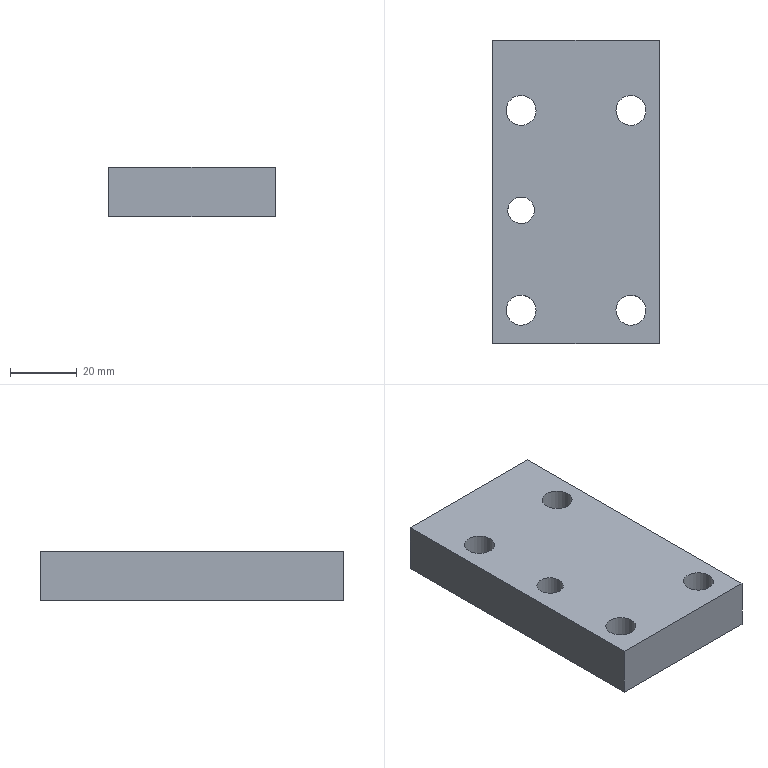Part | STEP file | SN10_006_005-02_PLACA | 1 solid | 11 faces | box 50 x 91 x 15 mm | volume 63679 mm3 | plane 6 | cylinder 5 | commonest cylinder face diameters 9 x4 8 x1
STEP:
#1=CARTESIAN_POINT('',(0.,0.,0.));
#2=DIRECTION('',(0.,0.,1.));
#3=DIRECTION('',(1.,0.,0.));
#4=AXIS2_PLACEMENT_3D('',#1,#2,#3);
#5=CARTESIAN_POINT('',(212.01,-237.918,73.5));
#6=VERTEX_POINT('',#5);
#7=CARTESIAN_POINT('',(208.5,-236.,73.5));
#8=DIRECTION('',(0.,0.,1.));
#9=DIRECTION('',(1.,0.,0.));
#10=AXIS2_PLACEMENT_3D('',#7,#8,#9);
#11=CIRCLE('',#10,4.);
#12=CARTESIAN_POINT('',(208.5,-236.,73.4));
#13=DIRECTION('',(0.,0.,-1.));
#14=DIRECTION('',(0.8776,-0.4794,0.));
#15=AXIS2_PLACEMENT_3D('',#12,#13,#14);
#16=CYLINDRICAL_SURFACE('',#15,4.);
#17=CARTESIAN_POINT('',(12.066,-0.1));
#18=DIRECTION('',(-1.,0.));
#19=VECTOR('',#18,1.);
#20=LINE('',#17,#19);
#21=(GEOMETRIC_REPRESENTATION_CONTEXT(2)PARAMETRIC_REPRESENTATION_CONTEXT()REPRESENTATION_CONTEXT('',''));
#22=DEFINITIONAL_REPRESENTATION('',(#20),#21);
#23=PCURVE('',#16,#22);
#24=CARTESIAN_POINT('',(200.,-185.,73.5));
#25=DIRECTION('',(0.,0.,1.));
#26=DIRECTION('',(1.,0.,0.));
#27=AXIS2_PLACEMENT_3D('',#24,#25,#26);
#28=PLANE('',#27);
#29=CARTESIAN_POINT('',(8.5,-51.));
#30=DIRECTION('',(1.,0.));
#31=AXIS2_PLACEMENT_2D('',#29,#30);
#32=CIRCLE('',#31,4.);
#33=(GEOMETRIC_REPRESENTATION_CONTEXT(2)PARAMETRIC_REPRESENTATION_CONTEXT()REPRESENTATION_CONTEXT('',''));
#34=DEFINITIONAL_REPRESENTATION('',(#32),#33);
#35=PCURVE('',#28,#34);
#36=SURFACE_CURVE('',#11,(#23,#35),.PCURVE_S1.);
#37=EDGE_CURVE('',#6,#6,#36,.T.);
#38=ORIENTED_EDGE('',*,*,#37,.F.);
#39=CARTESIAN_POINT('',(212.01,-237.918,58.5));
#40=VERTEX_POINT('',#39);
#41=CARTESIAN_POINT('',(212.01,-237.918,73.5));
#42=CARTESIAN_POINT('',(212.01,-237.918,58.5));
#43=B_SPLINE_CURVE_WITH_KNOTS('',1,(#41,#42),.UNSPECIFIED.,.F.,.F.,(2,2),(-0.1,14.9),.PIECEWISE_BEZIER_KNOTS.);
#44=CARTESIAN_POINT('',(6.283,0.));
#45=DIRECTION('',(0.,1.));
#46=VECTOR('',#45,1.);
#47=LINE('',#44,#46);
#48=(GEOMETRIC_REPRESENTATION_CONTEXT(2)PARAMETRIC_REPRESENTATION_CONTEXT()REPRESENTATION_CONTEXT('',''));
#49=DEFINITIONAL_REPRESENTATION('',(#47),#48);
#50=PCURVE('',#16,#49);
#51=CARTESIAN_POINT('',(0.,0.));
#52=DIRECTION('',(0.,1.));
#53=VECTOR('',#52,1.);
#54=LINE('',#51,#53);
#55=(GEOMETRIC_REPRESENTATION_CONTEXT(2)PARAMETRIC_REPRESENTATION_CONTEXT()REPRESENTATION_CONTEXT('',''));
#56=DEFINITIONAL_REPRESENTATION('',(#54),#55);
#57=PCURVE('',#16,#56);
#58=SEAM_CURVE('',#43,(#50,#57),.PCURVE_S1.);
#59=EDGE_CURVE('',#6,#40,#58,.T.);
#60=ORIENTED_EDGE('',*,*,#59,.T.);
#61=CARTESIAN_POINT('',(208.5,-236.,58.5));
#62=DIRECTION('',(0.,0.,-1.));
#63=DIRECTION('',(1.,0.,0.));
#64=AXIS2_PLACEMENT_3D('',#61,#62,#63);
#65=CIRCLE('',#64,4.);
#66=CARTESIAN_POINT('',(-0.5,14.9));
#67=DIRECTION('',(1.,0.));
#68=VECTOR('',#67,1.);
#69=LINE('',#66,#68);
#70=(GEOMETRIC_REPRESENTATION_CONTEXT(2)PARAMETRIC_REPRESENTATION_CONTEXT()REPRESENTATION_CONTEXT('',''));
#71=DEFINITIONAL_REPRESENTATION('',(#69),#70);
#72=PCURVE('',#16,#71);
#73=CARTESIAN_POINT('',(200.,-276.,58.5));
#74=DIRECTION('',(0.,0.,-1.));
#75=DIRECTION('',(-1.,0.,0.));
#76=AXIS2_PLACEMENT_3D('',#73,#74,#75);
#77=PLANE('',#76);
#78=CARTESIAN_POINT('',(-8.5,40.));
#79=DIRECTION('',(-1.,0.));
#80=AXIS2_PLACEMENT_2D('',#78,#79);
#81=CIRCLE('',#80,4.);
#82=(GEOMETRIC_REPRESENTATION_CONTEXT(2)PARAMETRIC_REPRESENTATION_CONTEXT()REPRESENTATION_CONTEXT('',''));
#83=DEFINITIONAL_REPRESENTATION('',(#81),#82);
#84=PCURVE('',#77,#83);
#85=SURFACE_CURVE('',#65,(#72,#84),.PCURVE_S1.);
#86=EDGE_CURVE('',#40,#40,#85,.T.);
#87=ORIENTED_EDGE('',*,*,#86,.F.);
#88=ORIENTED_EDGE('',*,*,#59,.F.);
#89=EDGE_LOOP('',(#38,#60,#87,#88));
#90=FACE_BOUND('',#89,.F.);
#91=ADVANCED_FACE('',(#90),#16,.F.);
#92=CARTESIAN_POINT('',(250.,-185.,73.5));
#93=VERTEX_POINT('',#92);
#94=CARTESIAN_POINT('',(250.,-276.,73.5));
#95=VERTEX_POINT('',#94);
#96=CARTESIAN_POINT('',(250.,-185.,73.5));
#97=DIRECTION('',(0.,-1.,0.));
#98=VECTOR('',#97,1.);
#99=LINE('',#96,#98);
#100=CARTESIAN_POINT('',(50.,0.));
#101=DIRECTION('',(0.,-1.));
#102=VECTOR('',#101,1.);
#103=LINE('',#100,#102);
#104=(GEOMETRIC_REPRESENTATION_CONTEXT(2)PARAMETRIC_REPRESENTATION_CONTEXT()REPRESENTATION_CONTEXT('',''));
#105=DEFINITIONAL_REPRESENTATION('',(#103),#104);
#106=PCURVE('',#28,#105);
#107=CARTESIAN_POINT('',(250.,0.,0.));
#108=DIRECTION('',(-1.,0.,0.));
#109=DIRECTION('',(0.,0.,1.));
#110=AXIS2_PLACEMENT_3D('',#107,#108,#109);
#111=PLANE('',#110);
#112=CARTESIAN_POINT('',(73.5,-185.));
#113=DIRECTION('',(0.,-1.));
#114=VECTOR('',#113,1.);
#115=LINE('',#112,#114);
#116=(GEOMETRIC_REPRESENTATION_CONTEXT(2)PARAMETRIC_REPRESENTATION_CONTEXT()REPRESENTATION_CONTEXT('',''));
#117=DEFINITIONAL_REPRESENTATION('',(#115),#116);
#118=PCURVE('',#111,#117);
#119=SURFACE_CURVE('',#99,(#106,#118),.PCURVE_S1.);
#120=EDGE_CURVE('',#93,#95,#119,.T.);
#121=ORIENTED_EDGE('',*,*,#120,.F.);
#122=CARTESIAN_POINT('',(200.,-185.,73.5));
#123=VERTEX_POINT('',#122);
#124=CARTESIAN_POINT('',(200.,-185.,73.5));
#125=DIRECTION('',(1.,0.,0.));
#126=VECTOR('',#125,1.);
#127=LINE('',#124,#126);
#128=CARTESIAN_POINT('',(0.,0.));
#129=DIRECTION('',(1.,0.));
#130=VECTOR('',#129,1.);
#131=LINE('',#128,#130);
#132=(GEOMETRIC_REPRESENTATION_CONTEXT(2)PARAMETRIC_REPRESENTATION_CONTEXT()REPRESENTATION_CONTEXT('',''));
#133=DEFINITIONAL_REPRESENTATION('',(#131),#132);
#134=PCURVE('',#28,#133);
#135=CARTESIAN_POINT('',(200.,-185.,73.5));
#136=DIRECTION('',(0.,-1.,0.));
#137=DIRECTION('',(0.,0.,-1.));
#138=AXIS2_PLACEMENT_3D('',#135,#136,#137);
#139=PLANE('',#138);
#140=CARTESIAN_POINT('',(0.,0.));
#141=DIRECTION('',(0.,1.));
#142=VECTOR('',#141,1.);
#143=LINE('',#140,#142);
#144=(GEOMETRIC_REPRESENTATION_CONTEXT(2)PARAMETRIC_REPRESENTATION_CONTEXT()REPRESENTATION_CONTEXT('',''));
#145=DEFINITIONAL_REPRESENTATION('',(#143),#144);
#146=PCURVE('',#139,#145);
#147=SURFACE_CURVE('',#127,(#134,#146),.PCURVE_S1.);
#148=EDGE_CURVE('',#123,#93,#147,.T.);
#149=ORIENTED_EDGE('',*,*,#148,.F.);
#150=CARTESIAN_POINT('',(200.,-276.,73.5));
#151=VERTEX_POINT('',#150);
#152=CARTESIAN_POINT('',(200.,-185.,73.5));
#153=DIRECTION('',(0.,-1.,0.));
#154=VECTOR('',#153,1.);
#155=LINE('',#152,#154);
#156=CARTESIAN_POINT('',(0.,0.));
#157=DIRECTION('',(0.,-1.));
#158=VECTOR('',#157,1.);
#159=LINE('',#156,#158);
#160=(GEOMETRIC_REPRESENTATION_CONTEXT(2)PARAMETRIC_REPRESENTATION_CONTEXT()REPRESENTATION_CONTEXT('',''));
#161=DEFINITIONAL_REPRESENTATION('',(#159),#160);
#162=PCURVE('',#28,#161);
#163=CARTESIAN_POINT('',(200.,0.,0.));
#164=DIRECTION('',(-1.,0.,0.));
#165=DIRECTION('',(0.,0.,1.));
#166=AXIS2_PLACEMENT_3D('',#163,#164,#165);
#167=PLANE('',#166);
#168=CARTESIAN_POINT('',(73.5,-185.));
#169=DIRECTION('',(0.,-1.));
#170=VECTOR('',#169,1.);
#171=LINE('',#168,#170);
#172=(GEOMETRIC_REPRESENTATION_CONTEXT(2)PARAMETRIC_REPRESENTATION_CONTEXT()REPRESENTATION_CONTEXT('',''));
#173=DEFINITIONAL_REPRESENTATION('',(#171),#172);
#174=PCURVE('',#167,#173);
#175=SURFACE_CURVE('',#155,(#162,#174),.PCURVE_S1.);
#176=EDGE_CURVE('',#123,#151,#175,.T.);
#177=ORIENTED_EDGE('',*,*,#176,.T.);
#178=CARTESIAN_POINT('',(200.,-276.,73.5));
#179=DIRECTION('',(1.,0.,0.));
#180=VECTOR('',#179,1.);
#181=LINE('',#178,#180);
#182=CARTESIAN_POINT('',(0.,-91.));
#183=DIRECTION('',(1.,0.));
#184=VECTOR('',#183,1.);
#185=LINE('',#182,#184);
#186=(GEOMETRIC_REPRESENTATION_CONTEXT(2)PARAMETRIC_REPRESENTATION_CONTEXT()REPRESENTATION_CONTEXT('',''));
#187=DEFINITIONAL_REPRESENTATION('',(#185),#186);
#188=PCURVE('',#28,#187);
#189=CARTESIAN_POINT('',(200.,-276.,58.5));
#190=DIRECTION('',(0.,1.,0.));
#191=DIRECTION('',(0.,0.,1.));
#192=AXIS2_PLACEMENT_3D('',#189,#190,#191);
#193=PLANE('',#192);
#194=CARTESIAN_POINT('',(15.,0.));
#195=DIRECTION('',(0.,1.));
#196=VECTOR('',#195,1.);
#197=LINE('',#194,#196);
#198=(GEOMETRIC_REPRESENTATION_CONTEXT(2)PARAMETRIC_REPRESENTATION_CONTEXT()REPRESENTATION_CONTEXT('',''));
#199=DEFINITIONAL_REPRESENTATION('',(#197),#198);
#200=PCURVE('',#193,#199);
#201=SURFACE_CURVE('',#181,(#188,#200),.PCURVE_S1.);
#202=EDGE_CURVE('',#151,#95,#201,.T.);
#203=ORIENTED_EDGE('',*,*,#202,.T.);
#204=EDGE_LOOP('',(#121,#149,#177,#203));
#205=FACE_BOUND('',#204,.T.);
#206=ORIENTED_EDGE('',*,*,#37,.F.);
#207=EDGE_LOOP('',(#206));
#208=FACE_BOUND('',#207,.T.);
#209=CARTESIAN_POINT('',(212.449,-268.157,73.5));
#210=VERTEX_POINT('',#209);
#211=CARTESIAN_POINT('',(208.5,-266.,73.5));
#212=DIRECTION('',(0.,0.,1.));
#213=DIRECTION('',(1.,0.,0.));
#214=AXIS2_PLACEMENT_3D('',#211,#212,#213);
#215=CIRCLE('',#214,4.5);
#216=CARTESIAN_POINT('',(8.5,-81.));
#217=DIRECTION('',(1.,0.));
#218=AXIS2_PLACEMENT_2D('',#216,#217);
#219=CIRCLE('',#218,4.5);
#220=(GEOMETRIC_REPRESENTATION_CONTEXT(2)PARAMETRIC_REPRESENTATION_CONTEXT()REPRESENTATION_CONTEXT('',''));
#221=DEFINITIONAL_REPRESENTATION('',(#219),#220);
#222=PCURVE('',#28,#221);
#223=CARTESIAN_POINT('',(208.5,-266.,73.4));
#224=DIRECTION('',(0.,0.,-1.));
#225=DIRECTION('',(0.8776,-0.4794,0.));
#226=AXIS2_PLACEMENT_3D('',#223,#224,#225);
#227=CYLINDRICAL_SURFACE('',#226,4.5);
#228=CARTESIAN_POINT('',(12.066,-0.1));
#229=DIRECTION('',(-1.,0.));
#230=VECTOR('',#229,1.);
#231=LINE('',#228,#230);
#232=(GEOMETRIC_REPRESENTATION_CONTEXT(2)PARAMETRIC_REPRESENTATION_CONTEXT()REPRESENTATION_CONTEXT('',''));
#233=DEFINITIONAL_REPRESENTATION('',(#231),#232);
#234=PCURVE('',#227,#233);
#235=SURFACE_CURVE('',#215,(#222,#234),.PCURVE_S1.);
#236=EDGE_CURVE('',#210,#210,#235,.T.);
#237=ORIENTED_EDGE('',*,*,#236,.F.);
#238=EDGE_LOOP('',(#237));
#239=FACE_BOUND('',#238,.T.);
#240=CARTESIAN_POINT('',(212.449,-208.157,73.5));
#241=VERTEX_POINT('',#240);
#242=CARTESIAN_POINT('',(208.5,-206.,73.5));
#243=DIRECTION('',(0.,0.,1.));
#244=DIRECTION('',(1.,0.,0.));
#245=AXIS2_PLACEMENT_3D('',#242,#243,#244);
#246=CIRCLE('',#245,4.5);
#247=CARTESIAN_POINT('',(8.5,-21.));
#248=DIRECTION('',(1.,0.));
#249=AXIS2_PLACEMENT_2D('',#247,#248);
#250=CIRCLE('',#249,4.5);
#251=(GEOMETRIC_REPRESENTATION_CONTEXT(2)PARAMETRIC_REPRESENTATION_CONTEXT()REPRESENTATION_CONTEXT('',''));
#252=DEFINITIONAL_REPRESENTATION('',(#250),#251);
#253=PCURVE('',#28,#252);
#254=CARTESIAN_POINT('',(208.5,-206.,73.4));
#255=DIRECTION('',(0.,0.,-1.));
#256=DIRECTION('',(0.8776,-0.4794,0.));
#257=AXIS2_PLACEMENT_3D('',#254,#255,#256);
#258=CYLINDRICAL_SURFACE('',#257,4.5);
#259=CARTESIAN_POINT('',(12.066,-0.1));
#260=DIRECTION('',(-1.,0.));
#261=VECTOR('',#260,1.);
#262=LINE('',#259,#261);
#263=(GEOMETRIC_REPRESENTATION_CONTEXT(2)PARAMETRIC_REPRESENTATION_CONTEXT()REPRESENTATION_CONTEXT('',''));
#264=DEFINITIONAL_REPRESENTATION('',(#262),#263);
#265=PCURVE('',#258,#264);
#266=SURFACE_CURVE('',#246,(#253,#265),.PCURVE_S1.);
#267=EDGE_CURVE('',#241,#241,#266,.T.);
#268=ORIENTED_EDGE('',*,*,#267,.F.);
#269=EDGE_LOOP('',(#268));
#270=FACE_BOUND('',#269,.T.);
#271=CARTESIAN_POINT('',(245.449,-268.157,73.5));
#272=VERTEX_POINT('',#271);
#273=CARTESIAN_POINT('',(241.5,-266.,73.5));
#274=DIRECTION('',(0.,0.,1.));
#275=DIRECTION('',(1.,0.,0.));
#276=AXIS2_PLACEMENT_3D('',#273,#274,#275);
#277=CIRCLE('',#276,4.5);
#278=CARTESIAN_POINT('',(41.5,-81.));
#279=DIRECTION('',(1.,0.));
#280=AXIS2_PLACEMENT_2D('',#278,#279);
#281=CIRCLE('',#280,4.5);
#282=(GEOMETRIC_REPRESENTATION_CONTEXT(2)PARAMETRIC_REPRESENTATION_CONTEXT()REPRESENTATION_CONTEXT('',''));
#283=DEFINITIONAL_REPRESENTATION('',(#281),#282);
#284=PCURVE('',#28,#283);
#285=CARTESIAN_POINT('',(241.5,-266.,73.4));
#286=DIRECTION('',(0.,0.,-1.));
#287=DIRECTION('',(0.8776,-0.4794,0.));
#288=AXIS2_PLACEMENT_3D('',#285,#286,#287);
#289=CYLINDRICAL_SURFACE('',#288,4.5);
#290=CARTESIAN_POINT('',(12.066,-0.1));
#291=DIRECTION('',(-1.,0.));
#292=VECTOR('',#291,1.);
#293=LINE('',#290,#292);
#294=(GEOMETRIC_REPRESENTATION_CONTEXT(2)PARAMETRIC_REPRESENTATION_CONTEXT()REPRESENTATION_CONTEXT('',''));
#295=DEFINITIONAL_REPRESENTATION('',(#293),#294);
#296=PCURVE('',#289,#295);
#297=SURFACE_CURVE('',#277,(#284,#296),.PCURVE_S1.);
#298=EDGE_CURVE('',#272,#272,#297,.T.);
#299=ORIENTED_EDGE('',*,*,#298,.F.);
#300=EDGE_LOOP('',(#299));
#301=FACE_BOUND('',#300,.T.);
#302=CARTESIAN_POINT('',(245.449,-208.157,73.5));
#303=VERTEX_POINT('',#302);
#304=CARTESIAN_POINT('',(241.5,-206.,73.5));
#305=DIRECTION('',(0.,0.,1.));
#306=DIRECTION('',(1.,0.,0.));
#307=AXIS2_PLACEMENT_3D('',#304,#305,#306);
#308=CIRCLE('',#307,4.5);
#309=CARTESIAN_POINT('',(41.5,-21.));
#310=DIRECTION('',(1.,0.));
#311=AXIS2_PLACEMENT_2D('',#309,#310);
#312=CIRCLE('',#311,4.5);
#313=(GEOMETRIC_REPRESENTATION_CONTEXT(2)PARAMETRIC_REPRESENTATION_CONTEXT()REPRESENTATION_CONTEXT('',''));
#314=DEFINITIONAL_REPRESENTATION('',(#312),#313);
#315=PCURVE('',#28,#314);
#316=CARTESIAN_POINT('',(241.5,-206.,73.4));
#317=DIRECTION('',(0.,0.,-1.));
#318=DIRECTION('',(0.8776,-0.4794,0.));
#319=AXIS2_PLACEMENT_3D('',#316,#317,#318);
#320=CYLINDRICAL_SURFACE('',#319,4.5);
#321=CARTESIAN_POINT('',(12.066,-0.1));
#322=DIRECTION('',(-1.,0.));
#323=VECTOR('',#322,1.);
#324=LINE('',#321,#323);
#325=(GEOMETRIC_REPRESENTATION_CONTEXT(2)PARAMETRIC_REPRESENTATION_CONTEXT()REPRESENTATION_CONTEXT('',''));
#326=DEFINITIONAL_REPRESENTATION('',(#324),#325);
#327=PCURVE('',#320,#326);
#328=SURFACE_CURVE('',#308,(#315,#327),.PCURVE_S1.);
#329=EDGE_CURVE('',#303,#303,#328,.T.);
#330=ORIENTED_EDGE('',*,*,#329,.F.);
#331=EDGE_LOOP('',(#330));
#332=FACE_BOUND('',#331,.T.);
#333=ADVANCED_FACE('',(#205,#208,#239,#270,#301,#332),#28,.T.);
#334=CARTESIAN_POINT('',(250.,-276.,58.5));
#335=VERTEX_POINT('',#334);
#336=CARTESIAN_POINT('',(250.,-185.,58.5));
#337=VERTEX_POINT('',#336);
#338=CARTESIAN_POINT('',(250.,-276.,58.5));
#339=DIRECTION('',(0.,1.,0.));
#340=VECTOR('',#339,1.);
#341=LINE('',#338,#340);
#342=CARTESIAN_POINT('',(-50.,0.));
#343=DIRECTION('',(0.,1.));
#344=VECTOR('',#343,1.);
#345=LINE('',#342,#344);
#346=(GEOMETRIC_REPRESENTATION_CONTEXT(2)PARAMETRIC_REPRESENTATION_CONTEXT()REPRESENTATION_CONTEXT('',''));
#347=DEFINITIONAL_REPRESENTATION('',(#345),#346);
#348=PCURVE('',#77,#347);
#349=CARTESIAN_POINT('',(58.5,-276.));
#350=DIRECTION('',(0.,1.));
#351=VECTOR('',#350,1.);
#352=LINE('',#349,#351);
#353=(GEOMETRIC_REPRESENTATION_CONTEXT(2)PARAMETRIC_REPRESENTATION_CONTEXT()REPRESENTATION_CONTEXT('',''));
#354=DEFINITIONAL_REPRESENTATION('',(#352),#353);
#355=PCURVE('',#111,#354);
#356=SURFACE_CURVE('',#341,(#348,#355),.PCURVE_S1.);
#357=EDGE_CURVE('',#335,#337,#356,.T.);
#358=ORIENTED_EDGE('',*,*,#357,.F.);
#359=CARTESIAN_POINT('',(200.,-276.,58.5));
#360=VERTEX_POINT('',#359);
#361=CARTESIAN_POINT('',(200.,-276.,58.5));
#362=DIRECTION('',(1.,0.,0.));
#363=VECTOR('',#362,1.);
#364=LINE('',#361,#363);
#365=CARTESIAN_POINT('',(0.,0.));
#366=DIRECTION('',(-1.,0.));
#367=VECTOR('',#366,1.);
#368=LINE('',#365,#367);
#369=(GEOMETRIC_REPRESENTATION_CONTEXT(2)PARAMETRIC_REPRESENTATION_CONTEXT()REPRESENTATION_CONTEXT('',''));
#370=DEFINITIONAL_REPRESENTATION('',(#368),#369);
#371=PCURVE('',#77,#370);
#372=CARTESIAN_POINT('',(0.,0.));
#373=DIRECTION('',(0.,1.));
#374=VECTOR('',#373,1.);
#375=LINE('',#372,#374);
#376=(GEOMETRIC_REPRESENTATION_CONTEXT(2)PARAMETRIC_REPRESENTATION_CONTEXT()REPRESENTATION_CONTEXT('',''));
#377=DEFINITIONAL_REPRESENTATION('',(#375),#376);
#378=PCURVE('',#193,#377);
#379=SURFACE_CURVE('',#364,(#371,#378),.PCURVE_S1.);
#380=EDGE_CURVE('',#360,#335,#379,.T.);
#381=ORIENTED_EDGE('',*,*,#380,.F.);
#382=CARTESIAN_POINT('',(200.,-185.,58.5));
#383=VERTEX_POINT('',#382);
#384=CARTESIAN_POINT('',(200.,-276.,58.5));
#385=DIRECTION('',(0.,1.,0.));
#386=VECTOR('',#385,1.);
#387=LINE('',#384,#386);
#388=CARTESIAN_POINT('',(0.,0.));
#389=DIRECTION('',(0.,1.));
#390=VECTOR('',#389,1.);
#391=LINE('',#388,#390);
#392=(GEOMETRIC_REPRESENTATION_CONTEXT(2)PARAMETRIC_REPRESENTATION_CONTEXT()REPRESENTATION_CONTEXT('',''));
#393=DEFINITIONAL_REPRESENTATION('',(#391),#392);
#394=PCURVE('',#77,#393);
#395=CARTESIAN_POINT('',(58.5,-276.));
#396=DIRECTION('',(0.,1.));
#397=VECTOR('',#396,1.);
#398=LINE('',#395,#397);
#399=(GEOMETRIC_REPRESENTATION_CONTEXT(2)PARAMETRIC_REPRESENTATION_CONTEXT()REPRESENTATION_CONTEXT('',''));
#400=DEFINITIONAL_REPRESENTATION('',(#398),#399);
#401=PCURVE('',#167,#400);
#402=SURFACE_CURVE('',#387,(#394,#401),.PCURVE_S1.);
#403=EDGE_CURVE('',#360,#383,#402,.T.);
#404=ORIENTED_EDGE('',*,*,#403,.T.);
#405=CARTESIAN_POINT('',(200.,-185.,58.5));
#406=DIRECTION('',(1.,0.,0.));
#407=VECTOR('',#406,1.);
#408=LINE('',#405,#407);
#409=CARTESIAN_POINT('',(0.,91.));
#410=DIRECTION('',(-1.,0.));
#411=VECTOR('',#410,1.);
#412=LINE('',#409,#411);
#413=(GEOMETRIC_REPRESENTATION_CONTEXT(2)PARAMETRIC_REPRESENTATION_CONTEXT()REPRESENTATION_CONTEXT('',''));
#414=DEFINITIONAL_REPRESENTATION('',(#412),#413);
#415=PCURVE('',#77,#414);
#416=CARTESIAN_POINT('',(15.,0.));
#417=DIRECTION('',(0.,1.));
#418=VECTOR('',#417,1.);
#419=LINE('',#416,#418);
#420=(GEOMETRIC_REPRESENTATION_CONTEXT(2)PARAMETRIC_REPRESENTATION_CONTEXT()REPRESENTATION_CONTEXT('',''));
#421=DEFINITIONAL_REPRESENTATION('',(#419),#420);
#422=PCURVE('',#139,#421);
#423=SURFACE_CURVE('',#408,(#415,#422),.PCURVE_S1.);
#424=EDGE_CURVE('',#383,#337,#423,.T.);
#425=ORIENTED_EDGE('',*,*,#424,.T.);
#426=EDGE_LOOP('',(#358,#381,#404,#425));
#427=FACE_BOUND('',#426,.T.);
#428=ORIENTED_EDGE('',*,*,#86,.F.);
#429=EDGE_LOOP('',(#428));
#430=FACE_BOUND('',#429,.T.);
#431=CARTESIAN_POINT('',(212.449,-268.157,58.5));
#432=VERTEX_POINT('',#431);
#433=CARTESIAN_POINT('',(208.5,-266.,58.5));
#434=DIRECTION('',(0.,0.,-1.));
#435=DIRECTION('',(1.,0.,0.));
#436=AXIS2_PLACEMENT_3D('',#433,#434,#435);
#437=CIRCLE('',#436,4.5);
#438=CARTESIAN_POINT('',(-8.5,10.));
#439=DIRECTION('',(-1.,0.));
#440=AXIS2_PLACEMENT_2D('',#438,#439);
#441=CIRCLE('',#440,4.5);
#442=(GEOMETRIC_REPRESENTATION_CONTEXT(2)PARAMETRIC_REPRESENTATION_CONTEXT()REPRESENTATION_CONTEXT('',''));
#443=DEFINITIONAL_REPRESENTATION('',(#441),#442);
#444=PCURVE('',#77,#443);
#445=CARTESIAN_POINT('',(-0.5,14.9));
#446=DIRECTION('',(1.,0.));
#447=VECTOR('',#446,1.);
#448=LINE('',#445,#447);
#449=(GEOMETRIC_REPRESENTATION_CONTEXT(2)PARAMETRIC_REPRESENTATION_CONTEXT()REPRESENTATION_CONTEXT('',''));
#450=DEFINITIONAL_REPRESENTATION('',(#448),#449);
#451=PCURVE('',#227,#450);
#452=SURFACE_CURVE('',#437,(#444,#451),.PCURVE_S1.);
#453=EDGE_CURVE('',#432,#432,#452,.T.);
#454=ORIENTED_EDGE('',*,*,#453,.F.);
#455=EDGE_LOOP('',(#454));
#456=FACE_BOUND('',#455,.T.);
#457=CARTESIAN_POINT('',(212.449,-208.157,58.5));
#458=VERTEX_POINT('',#457);
#459=CARTESIAN_POINT('',(208.5,-206.,58.5));
#460=DIRECTION('',(0.,0.,-1.));
#461=DIRECTION('',(1.,0.,0.));
#462=AXIS2_PLACEMENT_3D('',#459,#460,#461);
#463=CIRCLE('',#462,4.5);
#464=CARTESIAN_POINT('',(-8.5,70.));
#465=DIRECTION('',(-1.,0.));
#466=AXIS2_PLACEMENT_2D('',#464,#465);
#467=CIRCLE('',#466,4.5);
#468=(GEOMETRIC_REPRESENTATION_CONTEXT(2)PARAMETRIC_REPRESENTATION_CONTEXT()REPRESENTATION_CONTEXT('',''));
#469=DEFINITIONAL_REPRESENTATION('',(#467),#468);
#470=PCURVE('',#77,#469);
#471=CARTESIAN_POINT('',(-0.5,14.9));
#472=DIRECTION('',(1.,0.));
#473=VECTOR('',#472,1.);
#474=LINE('',#471,#473);
#475=(GEOMETRIC_REPRESENTATION_CONTEXT(2)PARAMETRIC_REPRESENTATION_CONTEXT()REPRESENTATION_CONTEXT('',''));
#476=DEFINITIONAL_REPRESENTATION('',(#474),#475);
#477=PCURVE('',#258,#476);
#478=SURFACE_CURVE('',#463,(#470,#477),.PCURVE_S1.);
#479=EDGE_CURVE('',#458,#458,#478,.T.);
#480=ORIENTED_EDGE('',*,*,#479,.F.);
#481=EDGE_LOOP('',(#480));
#482=FACE_BOUND('',#481,.T.);
#483=CARTESIAN_POINT('',(245.449,-268.157,58.5));
#484=VERTEX_POINT('',#483);
#485=CARTESIAN_POINT('',(241.5,-266.,58.5));
#486=DIRECTION('',(0.,0.,-1.));
#487=DIRECTION('',(1.,0.,0.));
#488=AXIS2_PLACEMENT_3D('',#485,#486,#487);
#489=CIRCLE('',#488,4.5);
#490=CARTESIAN_POINT('',(-41.5,10.));
#491=DIRECTION('',(-1.,0.));
#492=AXIS2_PLACEMENT_2D('',#490,#491);
#493=CIRCLE('',#492,4.5);
#494=(GEOMETRIC_REPRESENTATION_CONTEXT(2)PARAMETRIC_REPRESENTATION_CONTEXT()REPRESENTATION_CONTEXT('',''));
#495=DEFINITIONAL_REPRESENTATION('',(#493),#494);
#496=PCURVE('',#77,#495);
#497=CARTESIAN_POINT('',(-0.5,14.9));
#498=DIRECTION('',(1.,0.));
#499=VECTOR('',#498,1.);
#500=LINE('',#497,#499);
#501=(GEOMETRIC_REPRESENTATION_CONTEXT(2)PARAMETRIC_REPRESENTATION_CONTEXT()REPRESENTATION_CONTEXT('',''));
#502=DEFINITIONAL_REPRESENTATION('',(#500),#501);
#503=PCURVE('',#289,#502);
#504=SURFACE_CURVE('',#489,(#496,#503),.PCURVE_S1.);
#505=EDGE_CURVE('',#484,#484,#504,.T.);
#506=ORIENTED_EDGE('',*,*,#505,.F.);
#507=EDGE_LOOP('',(#506));
#508=FACE_BOUND('',#507,.T.);
#509=CARTESIAN_POINT('',(245.449,-208.157,58.5));
#510=VERTEX_POINT('',#509);
#511=CARTESIAN_POINT('',(241.5,-206.,58.5));
#512=DIRECTION('',(0.,0.,-1.));
#513=DIRECTION('',(1.,0.,0.));
#514=AXIS2_PLACEMENT_3D('',#511,#512,#513);
#515=CIRCLE('',#514,4.5);
#516=CARTESIAN_POINT('',(-41.5,70.));
#517=DIRECTION('',(-1.,0.));
#518=AXIS2_PLACEMENT_2D('',#516,#517);
#519=CIRCLE('',#518,4.5);
#520=(GEOMETRIC_REPRESENTATION_CONTEXT(2)PARAMETRIC_REPRESENTATION_CONTEXT()REPRESENTATION_CONTEXT('',''));
#521=DEFINITIONAL_REPRESENTATION('',(#519),#520);
#522=PCURVE('',#77,#521);
#523=CARTESIAN_POINT('',(-0.5,14.9));
#524=DIRECTION('',(1.,0.));
#525=VECTOR('',#524,1.);
#526=LINE('',#523,#525);
#527=(GEOMETRIC_REPRESENTATION_CONTEXT(2)PARAMETRIC_REPRESENTATION_CONTEXT()REPRESENTATION_CONTEXT('',''));
#528=DEFINITIONAL_REPRESENTATION('',(#526),#527);
#529=PCURVE('',#320,#528);
#530=SURFACE_CURVE('',#515,(#522,#529),.PCURVE_S1.);
#531=EDGE_CURVE('',#510,#510,#530,.T.);
#532=ORIENTED_EDGE('',*,*,#531,.F.);
#533=EDGE_LOOP('',(#532));
#534=FACE_BOUND('',#533,.T.);
#535=ADVANCED_FACE('',(#427,#430,#456,#482,#508,#534),#77,.T.);
#536=ORIENTED_EDGE('',*,*,#120,.T.);
#537=CARTESIAN_POINT('',(250.,-276.,58.5));
#538=DIRECTION('',(0.,0.,1.));
#539=VECTOR('',#538,1.);
#540=LINE('',#537,#539);
#541=CARTESIAN_POINT('',(58.5,-276.));
#542=DIRECTION('',(1.,0.));
#543=VECTOR('',#542,1.);
#544=LINE('',#541,#543);
#545=(GEOMETRIC_REPRESENTATION_CONTEXT(2)PARAMETRIC_REPRESENTATION_CONTEXT()REPRESENTATION_CONTEXT('',''));
#546=DEFINITIONAL_REPRESENTATION('',(#544),#545);
#547=PCURVE('',#111,#546);
#548=CARTESIAN_POINT('',(0.,50.));
#549=DIRECTION('',(1.,0.));
#550=VECTOR('',#549,1.);
#551=LINE('',#548,#550);
#552=(GEOMETRIC_REPRESENTATION_CONTEXT(2)PARAMETRIC_REPRESENTATION_CONTEXT()REPRESENTATION_CONTEXT('',''));
#553=DEFINITIONAL_REPRESENTATION('',(#551),#552);
#554=PCURVE('',#193,#553);
#555=SURFACE_CURVE('',#540,(#547,#554),.PCURVE_S1.);
#556=EDGE_CURVE('',#335,#95,#555,.T.);
#557=ORIENTED_EDGE('',*,*,#556,.F.);
#558=ORIENTED_EDGE('',*,*,#357,.T.);
#559=CARTESIAN_POINT('',(250.,-185.,73.5));
#560=DIRECTION('',(0.,0.,-1.));
#561=VECTOR('',#560,1.);
#562=LINE('',#559,#561);
#563=CARTESIAN_POINT('',(73.5,-185.));
#564=DIRECTION('',(-1.,0.));
#565=VECTOR('',#564,1.);
#566=LINE('',#563,#565);
#567=(GEOMETRIC_REPRESENTATION_CONTEXT(2)PARAMETRIC_REPRESENTATION_CONTEXT()REPRESENTATION_CONTEXT('',''));
#568=DEFINITIONAL_REPRESENTATION('',(#566),#567);
#569=PCURVE('',#111,#568);
#570=CARTESIAN_POINT('',(0.,50.));
#571=DIRECTION('',(1.,0.));
#572=VECTOR('',#571,1.);
#573=LINE('',#570,#572);
#574=(GEOMETRIC_REPRESENTATION_CONTEXT(2)PARAMETRIC_REPRESENTATION_CONTEXT()REPRESENTATION_CONTEXT('',''));
#575=DEFINITIONAL_REPRESENTATION('',(#573),#574);
#576=PCURVE('',#139,#575);
#577=SURFACE_CURVE('',#562,(#569,#576),.PCURVE_S1.);
#578=EDGE_CURVE('',#93,#337,#577,.T.);
#579=ORIENTED_EDGE('',*,*,#578,.F.);
#580=EDGE_LOOP('',(#536,#557,#558,#579));
#581=FACE_BOUND('',#580,.T.);
#582=ADVANCED_FACE('',(#581),#111,.F.);
#583=ORIENTED_EDGE('',*,*,#556,.T.);
#584=ORIENTED_EDGE('',*,*,#202,.F.);
#585=CARTESIAN_POINT('',(200.,-276.,58.5));
#586=DIRECTION('',(0.,0.,1.));
#587=VECTOR('',#586,1.);
#588=LINE('',#585,#587);
#589=CARTESIAN_POINT('',(0.,0.));
#590=DIRECTION('',(1.,0.));
#591=VECTOR('',#590,1.);
#592=LINE('',#589,#591);
#593=(GEOMETRIC_REPRESENTATION_CONTEXT(2)PARAMETRIC_REPRESENTATION_CONTEXT()REPRESENTATION_CONTEXT('',''));
#594=DEFINITIONAL_REPRESENTATION('',(#592),#593);
#595=PCURVE('',#193,#594);
#596=CARTESIAN_POINT('',(58.5,-276.));
#597=DIRECTION('',(1.,0.));
#598=VECTOR('',#597,1.);
#599=LINE('',#596,#598);
#600=(GEOMETRIC_REPRESENTATION_CONTEXT(2)PARAMETRIC_REPRESENTATION_CONTEXT()REPRESENTATION_CONTEXT('',''));
#601=DEFINITIONAL_REPRESENTATION('',(#599),#600);
#602=PCURVE('',#167,#601);
#603=SURFACE_CURVE('',#588,(#595,#602),.PCURVE_S1.);
#604=EDGE_CURVE('',#360,#151,#603,.T.);
#605=ORIENTED_EDGE('',*,*,#604,.F.);
#606=ORIENTED_EDGE('',*,*,#380,.T.);
#607=EDGE_LOOP('',(#583,#584,#605,#606));
#608=FACE_BOUND('',#607,.T.);
#609=ADVANCED_FACE('',(#608),#193,.F.);
#610=ORIENTED_EDGE('',*,*,#329,.F.);
#611=CARTESIAN_POINT('',(245.449,-208.157,73.5));
#612=CARTESIAN_POINT('',(245.449,-208.157,58.5));
#613=B_SPLINE_CURVE_WITH_KNOTS('',1,(#611,#612),.UNSPECIFIED.,.F.,.F.,(2,2),(-0.1,14.9),.PIECEWISE_BEZIER_KNOTS.);
#614=CARTESIAN_POINT('',(6.283,0.));
#615=DIRECTION('',(0.,1.));
#616=VECTOR('',#615,1.);
#617=LINE('',#614,#616);
#618=(GEOMETRIC_REPRESENTATION_CONTEXT(2)PARAMETRIC_REPRESENTATION_CONTEXT()REPRESENTATION_CONTEXT('',''));
#619=DEFINITIONAL_REPRESENTATION('',(#617),#618);
#620=PCURVE('',#320,#619);
#621=CARTESIAN_POINT('',(0.,0.));
#622=DIRECTION('',(0.,1.));
#623=VECTOR('',#622,1.);
#624=LINE('',#621,#623);
#625=(GEOMETRIC_REPRESENTATION_CONTEXT(2)PARAMETRIC_REPRESENTATION_CONTEXT()REPRESENTATION_CONTEXT('',''));
#626=DEFINITIONAL_REPRESENTATION('',(#624),#625);
#627=PCURVE('',#320,#626);
#628=SEAM_CURVE('',#613,(#620,#627),.PCURVE_S1.);
#629=EDGE_CURVE('',#303,#510,#628,.T.);
#630=ORIENTED_EDGE('',*,*,#629,.T.);
#631=ORIENTED_EDGE('',*,*,#531,.F.);
#632=ORIENTED_EDGE('',*,*,#629,.F.);
#633=EDGE_LOOP('',(#610,#630,#631,#632));
#634=FACE_BOUND('',#633,.F.);
#635=ADVANCED_FACE('',(#634),#320,.F.);
#636=ORIENTED_EDGE('',*,*,#298,.F.);
#637=CARTESIAN_POINT('',(245.449,-268.157,73.5));
#638=CARTESIAN_POINT('',(245.449,-268.157,58.5));
#639=B_SPLINE_CURVE_WITH_KNOTS('',1,(#637,#638),.UNSPECIFIED.,.F.,.F.,(2,2),(-0.1,14.9),.PIECEWISE_BEZIER_KNOTS.);
#640=CARTESIAN_POINT('',(6.283,0.));
#641=DIRECTION('',(0.,1.));
#642=VECTOR('',#641,1.);
#643=LINE('',#640,#642);
#644=(GEOMETRIC_REPRESENTATION_CONTEXT(2)PARAMETRIC_REPRESENTATION_CONTEXT()REPRESENTATION_CONTEXT('',''));
#645=DEFINITIONAL_REPRESENTATION('',(#643),#644);
#646=PCURVE('',#289,#645);
#647=CARTESIAN_POINT('',(0.,0.));
#648=DIRECTION('',(0.,1.));
#649=VECTOR('',#648,1.);
#650=LINE('',#647,#649);
#651=(GEOMETRIC_REPRESENTATION_CONTEXT(2)PARAMETRIC_REPRESENTATION_CONTEXT()REPRESENTATION_CONTEXT('',''));
#652=DEFINITIONAL_REPRESENTATION('',(#650),#651);
#653=PCURVE('',#289,#652);
#654=SEAM_CURVE('',#639,(#646,#653),.PCURVE_S1.);
#655=EDGE_CURVE('',#272,#484,#654,.T.);
#656=ORIENTED_EDGE('',*,*,#655,.T.);
#657=ORIENTED_EDGE('',*,*,#505,.F.);
#658=ORIENTED_EDGE('',*,*,#655,.F.);
#659=EDGE_LOOP('',(#636,#656,#657,#658));
#660=FACE_BOUND('',#659,.F.);
#661=ADVANCED_FACE('',(#660),#289,.F.);
#662=ORIENTED_EDGE('',*,*,#267,.F.);
#663=CARTESIAN_POINT('',(212.449,-208.157,73.5));
#664=CARTESIAN_POINT('',(212.449,-208.157,58.5));
#665=B_SPLINE_CURVE_WITH_KNOTS('',1,(#663,#664),.UNSPECIFIED.,.F.,.F.,(2,2),(-0.1,14.9),.PIECEWISE_BEZIER_KNOTS.);
#666=CARTESIAN_POINT('',(6.283,0.));
#667=DIRECTION('',(0.,1.));
#668=VECTOR('',#667,1.);
#669=LINE('',#666,#668);
#670=(GEOMETRIC_REPRESENTATION_CONTEXT(2)PARAMETRIC_REPRESENTATION_CONTEXT()REPRESENTATION_CONTEXT('',''));
#671=DEFINITIONAL_REPRESENTATION('',(#669),#670);
#672=PCURVE('',#258,#671);
#673=CARTESIAN_POINT('',(0.,0.));
#674=DIRECTION('',(0.,1.));
#675=VECTOR('',#674,1.);
#676=LINE('',#673,#675);
#677=(GEOMETRIC_REPRESENTATION_CONTEXT(2)PARAMETRIC_REPRESENTATION_CONTEXT()REPRESENTATION_CONTEXT('',''));
#678=DEFINITIONAL_REPRESENTATION('',(#676),#677);
#679=PCURVE('',#258,#678);
#680=SEAM_CURVE('',#665,(#672,#679),.PCURVE_S1.);
#681=EDGE_CURVE('',#241,#458,#680,.T.);
#682=ORIENTED_EDGE('',*,*,#681,.T.);
#683=ORIENTED_EDGE('',*,*,#479,.F.);
#684=ORIENTED_EDGE('',*,*,#681,.F.);
#685=EDGE_LOOP('',(#662,#682,#683,#684));
#686=FACE_BOUND('',#685,.F.);
#687=ADVANCED_FACE('',(#686),#258,.F.);
#688=ORIENTED_EDGE('',*,*,#236,.F.);
#689=CARTESIAN_POINT('',(212.449,-268.157,73.5));
#690=CARTESIAN_POINT('',(212.449,-268.157,58.5));
#691=B_SPLINE_CURVE_WITH_KNOTS('',1,(#689,#690),.UNSPECIFIED.,.F.,.F.,(2,2),(-0.1,14.9),.PIECEWISE_BEZIER_KNOTS.);
#692=CARTESIAN_POINT('',(6.283,0.));
#693=DIRECTION('',(0.,1.));
#694=VECTOR('',#693,1.);
#695=LINE('',#692,#694);
#696=(GEOMETRIC_REPRESENTATION_CONTEXT(2)PARAMETRIC_REPRESENTATION_CONTEXT()REPRESENTATION_CONTEXT('',''));
#697=DEFINITIONAL_REPRESENTATION('',(#695),#696);
#698=PCURVE('',#227,#697);
#699=CARTESIAN_POINT('',(0.,0.));
#700=DIRECTION('',(0.,1.));
#701=VECTOR('',#700,1.);
#702=LINE('',#699,#701);
#703=(GEOMETRIC_REPRESENTATION_CONTEXT(2)PARAMETRIC_REPRESENTATION_CONTEXT()REPRESENTATION_CONTEXT('',''));
#704=DEFINITIONAL_REPRESENTATION('',(#702),#703);
#705=PCURVE('',#227,#704);
#706=SEAM_CURVE('',#691,(#698,#705),.PCURVE_S1.);
#707=EDGE_CURVE('',#210,#432,#706,.T.);
#708=ORIENTED_EDGE('',*,*,#707,.T.);
#709=ORIENTED_EDGE('',*,*,#453,.F.);
#710=ORIENTED_EDGE('',*,*,#707,.F.);
#711=EDGE_LOOP('',(#688,#708,#709,#710));
#712=FACE_BOUND('',#711,.F.);
#713=ADVANCED_FACE('',(#712),#227,.F.);
#714=CARTESIAN_POINT('',(200.,-185.,73.5));
#715=DIRECTION('',(0.,0.,-1.));
#716=VECTOR('',#715,1.);
#717=LINE('',#714,#716);
#718=CARTESIAN_POINT('',(73.5,-185.));
#719=DIRECTION('',(-1.,0.));
#720=VECTOR('',#719,1.);
#721=LINE('',#718,#720);
#722=(GEOMETRIC_REPRESENTATION_CONTEXT(2)PARAMETRIC_REPRESENTATION_CONTEXT()REPRESENTATION_CONTEXT('',''));
#723=DEFINITIONAL_REPRESENTATION('',(#721),#722);
#724=PCURVE('',#167,#723);
#725=CARTESIAN_POINT('',(0.,0.));
#726=DIRECTION('',(1.,0.));
#727=VECTOR('',#726,1.);
#728=LINE('',#725,#727);
#729=(GEOMETRIC_REPRESENTATION_CONTEXT(2)PARAMETRIC_REPRESENTATION_CONTEXT()REPRESENTATION_CONTEXT('',''));
#730=DEFINITIONAL_REPRESENTATION('',(#728),#729);
#731=PCURVE('',#139,#730);
#732=SURFACE_CURVE('',#717,(#724,#731),.PCURVE_S1.);
#733=EDGE_CURVE('',#123,#383,#732,.T.);
#734=ORIENTED_EDGE('',*,*,#733,.T.);
#735=ORIENTED_EDGE('',*,*,#403,.F.);
#736=ORIENTED_EDGE('',*,*,#604,.T.);
#737=ORIENTED_EDGE('',*,*,#176,.F.);
#738=EDGE_LOOP('',(#734,#735,#736,#737));
#739=FACE_BOUND('',#738,.T.);
#740=ADVANCED_FACE('',(#739),#167,.T.);
#741=ORIENTED_EDGE('',*,*,#578,.T.);
#742=ORIENTED_EDGE('',*,*,#424,.F.);
#743=ORIENTED_EDGE('',*,*,#733,.F.);
#744=ORIENTED_EDGE('',*,*,#148,.T.);
#745=EDGE_LOOP('',(#741,#742,#743,#744));
#746=FACE_BOUND('',#745,.T.);
#747=ADVANCED_FACE('',(#746),#139,.F.);
#748=CLOSED_SHELL('',(#91,#333,#535,#582,#609,#635,#661,#687,#713,#740,#747));
#749=MANIFOLD_SOLID_BREP('',#748);
#750=(LENGTH_UNIT()NAMED_UNIT(*)SI_UNIT(.MILLI.,.METRE.));
#751=UNCERTAINTY_MEASURE_WITH_UNIT(LENGTH_MEASURE(0.000005),#750,'','');
#752=(NAMED_UNIT(*)PLANE_ANGLE_UNIT()SI_UNIT($,.RADIAN.));
#753=(NAMED_UNIT(*)SI_UNIT($,.STERADIAN.)SOLID_ANGLE_UNIT());
#754=(GEOMETRIC_REPRESENTATION_CONTEXT(3)GLOBAL_UNCERTAINTY_ASSIGNED_CONTEXT((#751))GLOBAL_UNIT_ASSIGNED_CONTEXT((#750,#752,#753))REPRESENTATION_CONTEXT('',''));
#755=ADVANCED_BREP_SHAPE_REPRESENTATION('',(#4,#749),#754);